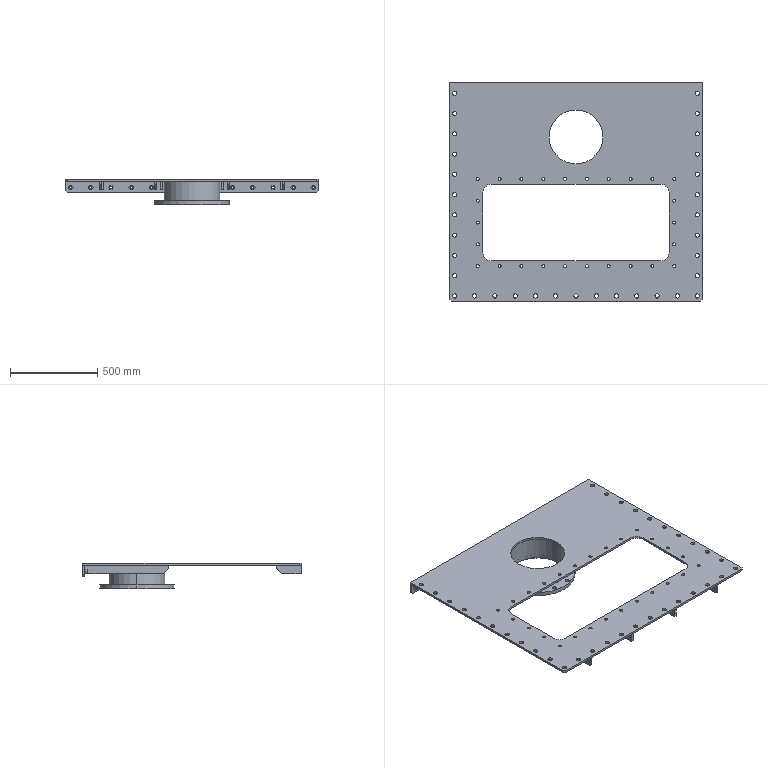Part | SolidWorks | features ICE 12, LPattern 7, Chamfer 4, MirrorPattern 2, MirrorSolid 2, Extrusion 1, Fillet 1, HoleWzd 1 | 25 solids | 392 faces | box 1448 x 1250 x 147 mm | volume 19462200 mm3 | cylinder 208 | plane 184 | commonest cylinder face diameters 24 x66 14 x52 17.5 x52 23 x24 100 x4 309 x2